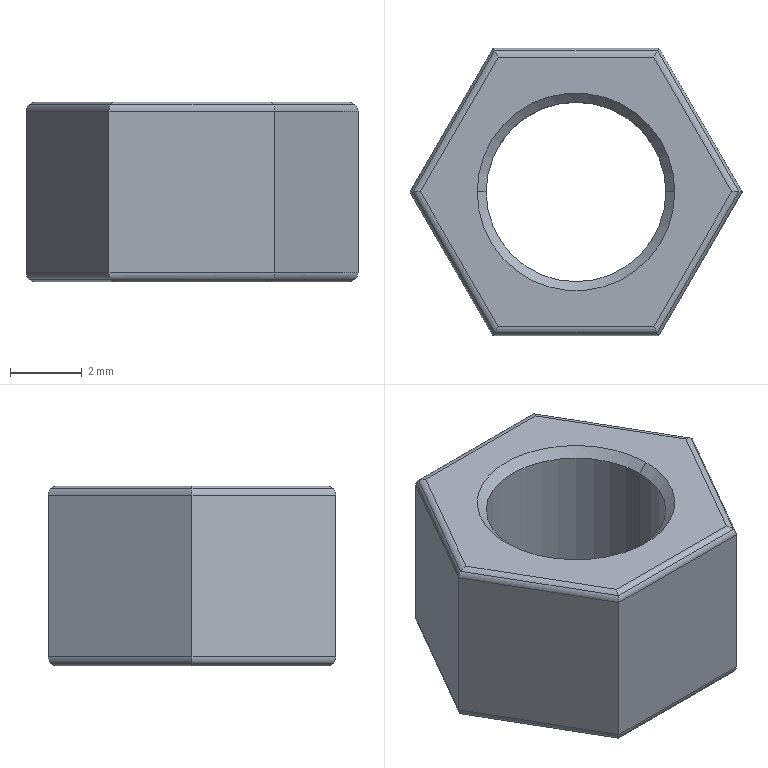Part | SolidWorks | features BaseBody 1 | 1 solid | 38 faces | box 9.238 x 8 x 5 mm | volume 177.206 mm3 | cylinder 26 | plane 8 | cone 4 | commonest cylinder face diameters 0.5 x24 5 x2
STEP:
#1=CARTESIAN_POINT('',(-2.5,0.,0.25));
#2=VERTEX_POINT('',#1);
#3=CARTESIAN_POINT('',(2.5,0.,0.25));
#4=VERTEX_POINT('',#3);
#5=CARTESIAN_POINT('',(0.,0.,0.25));
#6=DIRECTION('',(0.,0.,1.));
#7=DIRECTION('',(-1.,0.,0.));
#8=AXIS2_PLACEMENT_3D('',#5,#6,#7);
#9=CIRCLE('',#8,2.5);
#10=EDGE_CURVE('',#2,#4,#9,.T.);
#11=ORIENTED_EDGE('',*,*,#10,.T.);
#12=CARTESIAN_POINT('',(2.75,0.,0.));
#13=VERTEX_POINT('',#12);
#14=CARTESIAN_POINT('',(2.625,0.,0.125));
#15=DIRECTION('',(0.7071,0.,-0.7071));
#16=VECTOR('',#15,1000.);
#17=LINE('',#14,#16);
#18=EDGE_CURVE('',#4,#13,#17,.T.);
#19=ORIENTED_EDGE('',*,*,#18,.T.);
#20=CARTESIAN_POINT('',(-2.75,0.,0.));
#21=VERTEX_POINT('',#20);
#22=CARTESIAN_POINT('',(0.,0.,0.));
#23=DIRECTION('',(0.,0.,-1.));
#24=DIRECTION('',(-1.,0.,0.));
#25=AXIS2_PLACEMENT_3D('',#22,#23,#24);
#26=CIRCLE('',#25,2.75);
#27=EDGE_CURVE('',#13,#21,#26,.T.);
#28=ORIENTED_EDGE('',*,*,#27,.T.);
#29=CARTESIAN_POINT('',(-2.625,0.,0.125));
#30=DIRECTION('',(-0.7071,0.,-0.7071));
#31=VECTOR('',#30,1000.);
#32=LINE('',#29,#31);
#33=EDGE_CURVE('',#2,#21,#32,.T.);
#34=ORIENTED_EDGE('',*,*,#33,.F.);
#35=EDGE_LOOP('',(#11,#19,#28,#34));
#36=FACE_OUTER_BOUND('',#35,.T.);
#37=CARTESIAN_POINT('',(0.,0.,0.125));
#38=DIRECTION('',(0.,0.,-1.));
#39=DIRECTION('',(-1.,0.,0.));
#40=AXIS2_PLACEMENT_3D('',#37,#38,#39);
#41=CONICAL_SURFACE('',#40,2.625,0.7854);
#42=ADVANCED_FACE('',(#36),#41,.F.);
#43=CARTESIAN_POINT('',(2.5,0.,4.75));
#44=VERTEX_POINT('',#43);
#45=CARTESIAN_POINT('',(-2.5,0.,4.75));
#46=VERTEX_POINT('',#45);
#47=CARTESIAN_POINT('',(0.,0.,4.75));
#48=DIRECTION('',(0.,0.,-1.));
#49=DIRECTION('',(-1.,0.,0.));
#50=AXIS2_PLACEMENT_3D('',#47,#48,#49);
#51=CIRCLE('',#50,2.5);
#52=EDGE_CURVE('',#44,#46,#51,.T.);
#53=ORIENTED_EDGE('',*,*,#52,.F.);
#54=CARTESIAN_POINT('',(2.5,0.,0.));
#55=DIRECTION('',(0.,0.,-1.));
#56=VECTOR('',#55,1000.);
#57=LINE('',#54,#56);
#58=EDGE_CURVE('',#44,#4,#57,.T.);
#59=ORIENTED_EDGE('',*,*,#58,.T.);
#60=ORIENTED_EDGE('',*,*,#10,.F.);
#61=CARTESIAN_POINT('',(-2.5,0.,0.));
#62=DIRECTION('',(0.,0.,-1.));
#63=VECTOR('',#62,1000.);
#64=LINE('',#61,#63);
#65=EDGE_CURVE('',#46,#2,#64,.T.);
#66=ORIENTED_EDGE('',*,*,#65,.F.);
#67=EDGE_LOOP('',(#53,#59,#60,#66));
#68=FACE_OUTER_BOUND('',#67,.T.);
#69=CARTESIAN_POINT('',(0.,0.,0.));
#70=DIRECTION('',(0.,0.,-1.));
#71=DIRECTION('',(-1.,0.,0.));
#72=AXIS2_PLACEMENT_3D('',#69,#70,#71);
#73=CYLINDRICAL_SURFACE('',#72,2.5);
#74=ADVANCED_FACE('',(#68),#73,.F.);
#75=CARTESIAN_POINT('',(0.,0.,4.75));
#76=DIRECTION('',(0.,0.,-1.));
#77=DIRECTION('',(-1.,0.,0.));
#78=AXIS2_PLACEMENT_3D('',#75,#76,#77);
#79=CIRCLE('',#78,2.5);
#80=EDGE_CURVE('',#46,#44,#79,.T.);
#81=ORIENTED_EDGE('',*,*,#80,.T.);
#82=CARTESIAN_POINT('',(2.75,0.,5.));
#83=VERTEX_POINT('',#82);
#84=CARTESIAN_POINT('',(2.625,0.,4.875));
#85=DIRECTION('',(0.7071,0.,0.7071));
#86=VECTOR('',#85,1000.);
#87=LINE('',#84,#86);
#88=EDGE_CURVE('',#44,#83,#87,.T.);
#89=ORIENTED_EDGE('',*,*,#88,.T.);
#90=CARTESIAN_POINT('',(-2.75,0.,5.));
#91=VERTEX_POINT('',#90);
#92=CARTESIAN_POINT('',(0.,0.,5.));
#93=DIRECTION('',(0.,0.,1.));
#94=DIRECTION('',(-1.,0.,0.));
#95=AXIS2_PLACEMENT_3D('',#92,#93,#94);
#96=CIRCLE('',#95,2.75);
#97=EDGE_CURVE('',#83,#91,#96,.T.);
#98=ORIENTED_EDGE('',*,*,#97,.T.);
#99=CARTESIAN_POINT('',(-2.625,0.,4.875));
#100=DIRECTION('',(-0.7071,0.,0.7071));
#101=VECTOR('',#100,1000.);
#102=LINE('',#99,#101);
#103=EDGE_CURVE('',#46,#91,#102,.T.);
#104=ORIENTED_EDGE('',*,*,#103,.F.);
#105=EDGE_LOOP('',(#81,#89,#98,#104));
#106=FACE_OUTER_BOUND('',#105,.T.);
#107=CARTESIAN_POINT('',(0.,0.,4.875));
#108=DIRECTION('',(0.,0.,1.));
#109=DIRECTION('',(-1.,0.,0.));
#110=AXIS2_PLACEMENT_3D('',#107,#108,#109);
#111=CONICAL_SURFACE('',#110,2.625,0.7854);
#112=ADVANCED_FACE('',(#106),#111,.F.);
#113=CARTESIAN_POINT('',(2.309,4.,0.25));
#114=VERTEX_POINT('',#113);
#115=CARTESIAN_POINT('',(2.267,3.927,0.07322));
#116=VERTEX_POINT('',#115);
#117=CARTESIAN_POINT('',(2.309,4.,0.25));
#118=CARTESIAN_POINT('',(2.309,4.,0.1828));
#119=CARTESIAN_POINT('',(2.295,3.974,0.1207));
#120=CARTESIAN_POINT('',(2.267,3.927,0.07322));
#121=(BOUNDED_CURVE()B_SPLINE_CURVE(3,(#117,#118,#119,#120),.UNSPECIFIED.,.F.,.T.)B_SPLINE_CURVE_WITH_KNOTS((4,4),(3.142,3.927),.UNSPECIFIED.)CURVE()GEOMETRIC_REPRESENTATION_ITEM()RATIONAL_B_SPLINE_CURVE((1.,0.9493,0.9493,1.))REPRESENTATION_ITEM(''));
#122=EDGE_CURVE('',#114,#116,#121,.T.);
#123=ORIENTED_EDGE('',*,*,#122,.T.);
#124=CARTESIAN_POINT('',(-2.267,3.927,0.07322));
#125=VERTEX_POINT('',#124);
#126=CARTESIAN_POINT('',(1.155,3.927,0.07322));
#127=DIRECTION('',(-1.,0.,0.));
#128=VECTOR('',#127,1000.);
#129=LINE('',#126,#128);
#130=EDGE_CURVE('',#116,#125,#129,.T.);
#131=ORIENTED_EDGE('',*,*,#130,.T.);
#132=CARTESIAN_POINT('',(-2.309,4.,0.25));
#133=VERTEX_POINT('',#132);
#134=CARTESIAN_POINT('',(-2.309,4.,0.25));
#135=CARTESIAN_POINT('',(-2.309,4.,0.1828));
#136=CARTESIAN_POINT('',(-2.295,3.974,0.1207));
#137=CARTESIAN_POINT('',(-2.267,3.927,0.07322));
#138=(BOUNDED_CURVE()B_SPLINE_CURVE(3,(#134,#135,#136,#137),.UNSPECIFIED.,.F.,.F.)B_SPLINE_CURVE_WITH_KNOTS((4,4),(3.142,3.927),.UNSPECIFIED.)CURVE()GEOMETRIC_REPRESENTATION_ITEM()RATIONAL_B_SPLINE_CURVE((1.,0.9493,0.9493,1.))REPRESENTATION_ITEM(''));
#139=EDGE_CURVE('',#133,#125,#138,.T.);
#140=ORIENTED_EDGE('',*,*,#139,.F.);
#141=CARTESIAN_POINT('',(1.155,4.,0.25));
#142=DIRECTION('',(1.,0.,0.));
#143=VECTOR('',#142,1000.);
#144=LINE('',#141,#143);
#145=EDGE_CURVE('',#133,#114,#144,.T.);
#146=ORIENTED_EDGE('',*,*,#145,.T.);
#147=EDGE_LOOP('',(#123,#131,#140,#146));
#148=FACE_OUTER_BOUND('',#147,.T.);
#149=CARTESIAN_POINT('',(1.155,3.75,0.25));
#150=DIRECTION('',(-1.,0.,0.));
#151=DIRECTION('',(0.,0.7071,-0.7071));
#152=AXIS2_PLACEMENT_3D('',#149,#150,#151);
#153=CYLINDRICAL_SURFACE('',#152,0.25);
#154=ADVANCED_FACE('',(#148),#153,.T.);
#155=CARTESIAN_POINT('',(-2.309,-4.,0.25));
#156=VERTEX_POINT('',#155);
#157=CARTESIAN_POINT('',(-2.267,-3.927,0.07322));
#158=VERTEX_POINT('',#157);
#159=CARTESIAN_POINT('',(-2.309,-4.,0.25));
#160=CARTESIAN_POINT('',(-2.309,-4.,0.1828));
#161=CARTESIAN_POINT('',(-2.295,-3.974,0.1207));
#162=CARTESIAN_POINT('',(-2.267,-3.927,0.07322));
#163=(BOUNDED_CURVE()B_SPLINE_CURVE(3,(#159,#160,#161,#162),.UNSPECIFIED.,.F.,.F.)B_SPLINE_CURVE_WITH_KNOTS((4,4),(3.142,3.927),.UNSPECIFIED.)CURVE()GEOMETRIC_REPRESENTATION_ITEM()RATIONAL_B_SPLINE_CURVE((1.,0.9493,0.9493,1.))REPRESENTATION_ITEM(''));
#164=EDGE_CURVE('',#156,#158,#163,.T.);
#165=ORIENTED_EDGE('',*,*,#164,.T.);
#166=CARTESIAN_POINT('',(2.267,-3.927,0.07322));
#167=VERTEX_POINT('',#166);
#168=CARTESIAN_POINT('',(-1.155,-3.927,0.07322));
#169=DIRECTION('',(1.,0.,0.));
#170=VECTOR('',#169,1000.);
#171=LINE('',#168,#170);
#172=EDGE_CURVE('',#158,#167,#171,.T.);
#173=ORIENTED_EDGE('',*,*,#172,.T.);
#174=CARTESIAN_POINT('',(2.309,-4.,0.25));
#175=VERTEX_POINT('',#174);
#176=CARTESIAN_POINT('',(2.267,-3.927,0.07322));
#177=CARTESIAN_POINT('',(2.295,-3.974,0.1207));
#178=CARTESIAN_POINT('',(2.309,-4.,0.1828));
#179=CARTESIAN_POINT('',(2.309,-4.,0.25));
#180=(BOUNDED_CURVE()B_SPLINE_CURVE(3,(#176,#177,#178,#179),.UNSPECIFIED.,.F.,.F.)B_SPLINE_CURVE_WITH_KNOTS((4,4),(5.498,6.283),.UNSPECIFIED.)CURVE()GEOMETRIC_REPRESENTATION_ITEM()RATIONAL_B_SPLINE_CURVE((1.,0.9493,0.9493,1.))REPRESENTATION_ITEM(''));
#181=EDGE_CURVE('',#167,#175,#180,.T.);
#182=ORIENTED_EDGE('',*,*,#181,.T.);
#183=CARTESIAN_POINT('',(-1.155,-4.,0.25));
#184=DIRECTION('',(-1.,0.,0.));
#185=VECTOR('',#184,1000.);
#186=LINE('',#183,#185);
#187=EDGE_CURVE('',#175,#156,#186,.T.);
#188=ORIENTED_EDGE('',*,*,#187,.T.);
#189=EDGE_LOOP('',(#165,#173,#182,#188));
#190=FACE_OUTER_BOUND('',#189,.T.);
#191=CARTESIAN_POINT('',(-1.155,-3.75,0.25));
#192=DIRECTION('',(1.,0.,0.));
#193=DIRECTION('',(0.,-0.7071,-0.7071));
#194=AXIS2_PLACEMENT_3D('',#191,#192,#193);
#195=CYLINDRICAL_SURFACE('',#194,0.25);
#196=ADVANCED_FACE('',(#190),#195,.T.);
#197=CARTESIAN_POINT('',(4.619,0.,0.25));
#198=VERTEX_POINT('',#197);
#199=CARTESIAN_POINT('',(4.534,0.,0.07322));
#200=VERTEX_POINT('',#199);
#201=CARTESIAN_POINT('',(4.619,0.,0.25));
#202=CARTESIAN_POINT('',(4.619,0.,0.1828));
#203=CARTESIAN_POINT('',(4.589,0.,0.1207));
#204=CARTESIAN_POINT('',(4.534,0.,0.07322));
#205=(BOUNDED_CURVE()B_SPLINE_CURVE(3,(#201,#202,#203,#204),.UNSPECIFIED.,.F.,.F.)B_SPLINE_CURVE_WITH_KNOTS((4,4),(3.142,3.927),.UNSPECIFIED.)CURVE()GEOMETRIC_REPRESENTATION_ITEM()RATIONAL_B_SPLINE_CURVE((1.,0.9493,0.9493,1.))REPRESENTATION_ITEM(''));
#206=EDGE_CURVE('',#198,#200,#205,.T.);
#207=ORIENTED_EDGE('',*,*,#206,.T.);
#208=CARTESIAN_POINT('',(3.978,0.9634,0.07322));
#209=DIRECTION('',(-0.5,0.866,0.));
#210=VECTOR('',#209,1000.);
#211=LINE('',#208,#210);
#212=EDGE_CURVE('',#200,#116,#211,.T.);
#213=ORIENTED_EDGE('',*,*,#212,.T.);
#214=ORIENTED_EDGE('',*,*,#122,.F.);
#215=CARTESIAN_POINT('',(4.041,1.,0.25));
#216=DIRECTION('',(0.5,-0.866,0.));
#217=VECTOR('',#216,1000.);
#218=LINE('',#215,#217);
#219=EDGE_CURVE('',#114,#198,#218,.T.);
#220=ORIENTED_EDGE('',*,*,#219,.T.);
#221=EDGE_LOOP('',(#207,#213,#214,#220));
#222=FACE_OUTER_BOUND('',#221,.T.);
#223=CARTESIAN_POINT('',(3.825,0.875,0.25));
#224=DIRECTION('',(-0.5,0.866,0.));
#225=DIRECTION('',(0.6124,0.3536,-0.7071));
#226=AXIS2_PLACEMENT_3D('',#223,#224,#225);
#227=CYLINDRICAL_SURFACE('',#226,0.25);
#228=ADVANCED_FACE('',(#222),#227,.T.);
#229=ORIENTED_EDGE('',*,*,#181,.F.);
#230=CARTESIAN_POINT('',(2.823,-2.963,0.07322));
#231=DIRECTION('',(0.5,0.866,0.));
#232=VECTOR('',#231,1000.);
#233=LINE('',#230,#232);
#234=EDGE_CURVE('',#167,#200,#233,.T.);
#235=ORIENTED_EDGE('',*,*,#234,.T.);
#236=ORIENTED_EDGE('',*,*,#206,.F.);
#237=CARTESIAN_POINT('',(2.887,-3.,0.25));
#238=DIRECTION('',(-0.5,-0.866,0.));
#239=VECTOR('',#238,1000.);
#240=LINE('',#237,#239);
#241=EDGE_CURVE('',#198,#175,#240,.T.);
#242=ORIENTED_EDGE('',*,*,#241,.T.);
#243=EDGE_LOOP('',(#229,#235,#236,#242));
#244=FACE_OUTER_BOUND('',#243,.T.);
#245=CARTESIAN_POINT('',(2.67,-2.875,0.25));
#246=DIRECTION('',(0.5,0.866,0.));
#247=DIRECTION('',(0.6124,-0.3536,-0.7071));
#248=AXIS2_PLACEMENT_3D('',#245,#246,#247);
#249=CYLINDRICAL_SURFACE('',#248,0.25);
#250=ADVANCED_FACE('',(#244),#249,.T.);
#251=CARTESIAN_POINT('',(-4.619,0.,0.25));
#252=VERTEX_POINT('',#251);
#253=CARTESIAN_POINT('',(-4.534,0.,0.07322));
#254=VERTEX_POINT('',#253);
#255=CARTESIAN_POINT('',(-4.619,0.,0.25));
#256=CARTESIAN_POINT('',(-4.619,0.,0.1828));
#257=CARTESIAN_POINT('',(-4.589,0.,0.1207));
#258=CARTESIAN_POINT('',(-4.534,0.,0.07322));
#259=(BOUNDED_CURVE()B_SPLINE_CURVE(3,(#255,#256,#257,#258),.UNSPECIFIED.,.F.,.T.)B_SPLINE_CURVE_WITH_KNOTS((4,4),(3.142,3.927),.UNSPECIFIED.)CURVE()GEOMETRIC_REPRESENTATION_ITEM()RATIONAL_B_SPLINE_CURVE((1.,0.9493,0.9493,1.))REPRESENTATION_ITEM(''));
#260=EDGE_CURVE('',#252,#254,#259,.T.);
#261=ORIENTED_EDGE('',*,*,#260,.T.);
#262=CARTESIAN_POINT('',(-3.978,-0.9634,0.07322));
#263=DIRECTION('',(0.5,-0.866,0.));
#264=VECTOR('',#263,1000.);
#265=LINE('',#262,#264);
#266=EDGE_CURVE('',#254,#158,#265,.T.);
#267=ORIENTED_EDGE('',*,*,#266,.T.);
#268=ORIENTED_EDGE('',*,*,#164,.F.);
#269=CARTESIAN_POINT('',(-4.041,-1.,0.25));
#270=DIRECTION('',(-0.5,0.866,0.));
#271=VECTOR('',#270,1000.);
#272=LINE('',#269,#271);
#273=EDGE_CURVE('',#156,#252,#272,.T.);
#274=ORIENTED_EDGE('',*,*,#273,.T.);
#275=EDGE_LOOP('',(#261,#267,#268,#274));
#276=FACE_OUTER_BOUND('',#275,.T.);
#277=CARTESIAN_POINT('',(-3.825,-0.875,0.25));
#278=DIRECTION('',(0.5,-0.866,0.));
#279=DIRECTION('',(-0.6124,-0.3536,-0.7071));
#280=AXIS2_PLACEMENT_3D('',#277,#278,#279);
#281=CYLINDRICAL_SURFACE('',#280,0.25);
#282=ADVANCED_FACE('',(#276),#281,.T.);
#283=ORIENTED_EDGE('',*,*,#139,.T.);
#284=CARTESIAN_POINT('',(-2.823,2.963,0.07322));
#285=DIRECTION('',(-0.5,-0.866,0.));
#286=VECTOR('',#285,1000.);
#287=LINE('',#284,#286);
#288=EDGE_CURVE('',#125,#254,#287,.T.);
#289=ORIENTED_EDGE('',*,*,#288,.T.);
#290=ORIENTED_EDGE('',*,*,#260,.F.);
#291=CARTESIAN_POINT('',(-2.887,3.,0.25));
#292=DIRECTION('',(0.5,0.866,0.));
#293=VECTOR('',#292,1000.);
#294=LINE('',#291,#293);
#295=EDGE_CURVE('',#252,#133,#294,.T.);
#296=ORIENTED_EDGE('',*,*,#295,.T.);
#297=EDGE_LOOP('',(#283,#289,#290,#296));
#298=FACE_OUTER_BOUND('',#297,.T.);
#299=CARTESIAN_POINT('',(-2.67,2.875,0.25));
#300=DIRECTION('',(-0.5,-0.866,0.));
#301=DIRECTION('',(-0.6124,0.3536,-0.7071));
#302=AXIS2_PLACEMENT_3D('',#299,#300,#301);
#303=CYLINDRICAL_SURFACE('',#302,0.25);
#304=ADVANCED_FACE('',(#298),#303,.T.);
#305=CARTESIAN_POINT('',(2.267,-3.927,4.927));
#306=VERTEX_POINT('',#305);
#307=CARTESIAN_POINT('',(2.309,-4.,4.75));
#308=VERTEX_POINT('',#307);
#309=CARTESIAN_POINT('',(2.267,-3.927,4.927));
#310=CARTESIAN_POINT('',(2.295,-3.974,4.879));
#311=CARTESIAN_POINT('',(2.309,-4.,4.817));
#312=CARTESIAN_POINT('',(2.309,-4.,4.75));
#313=(BOUNDED_CURVE()B_SPLINE_CURVE(3,(#309,#310,#311,#312),.UNSPECIFIED.,.F.,.F.)B_SPLINE_CURVE_WITH_KNOTS((4,4),(5.498,6.283),.UNSPECIFIED.)CURVE()GEOMETRIC_REPRESENTATION_ITEM()RATIONAL_B_SPLINE_CURVE((1.,0.9493,0.9493,1.))REPRESENTATION_ITEM(''));
#314=EDGE_CURVE('',#306,#308,#313,.T.);
#315=ORIENTED_EDGE('',*,*,#314,.F.);
#316=CARTESIAN_POINT('',(-2.267,-3.927,4.927));
#317=VERTEX_POINT('',#316);
#318=CARTESIAN_POINT('',(-1.155,-3.927,4.927));
#319=DIRECTION('',(-1.,0.,0.));
#320=VECTOR('',#319,1000.);
#321=LINE('',#318,#320);
#322=EDGE_CURVE('',#306,#317,#321,.T.);
#323=ORIENTED_EDGE('',*,*,#322,.T.);
#324=CARTESIAN_POINT('',(-2.309,-4.,4.75));
#325=VERTEX_POINT('',#324);
#326=CARTESIAN_POINT('',(-2.267,-3.927,4.927));
#327=CARTESIAN_POINT('',(-2.295,-3.974,4.879));
#328=CARTESIAN_POINT('',(-2.309,-4.,4.817));
#329=CARTESIAN_POINT('',(-2.309,-4.,4.75));
#330=(BOUNDED_CURVE()B_SPLINE_CURVE(3,(#326,#327,#328,#329),.UNSPECIFIED.,.F.,.F.)B_SPLINE_CURVE_WITH_KNOTS((4,4),(5.498,6.283),.UNSPECIFIED.)CURVE()GEOMETRIC_REPRESENTATION_ITEM()RATIONAL_B_SPLINE_CURVE((1.,0.9493,0.9493,1.))REPRESENTATION_ITEM(''));
#331=EDGE_CURVE('',#317,#325,#330,.T.);
#332=ORIENTED_EDGE('',*,*,#331,.T.);
#333=CARTESIAN_POINT('',(-1.155,-4.,4.75));
#334=DIRECTION('',(1.,0.,0.));
#335=VECTOR('',#334,1000.);
#336=LINE('',#333,#335);
#337=EDGE_CURVE('',#325,#308,#336,.T.);
#338=ORIENTED_EDGE('',*,*,#337,.T.);
#339=EDGE_LOOP('',(#315,#323,#332,#338));
#340=FACE_OUTER_BOUND('',#339,.T.);
#341=CARTESIAN_POINT('',(-1.155,-3.75,4.75));
#342=DIRECTION('',(-1.,0.,0.));
#343=DIRECTION('',(0.,-0.7071,0.7071));
#344=AXIS2_PLACEMENT_3D('',#341,#342,#343);
#345=CYLINDRICAL_SURFACE('',#344,0.25);
#346=ADVANCED_FACE('',(#340),#345,.T.);
#347=ORIENTED_EDGE('',*,*,#331,.F.);
#348=CARTESIAN_POINT('',(-4.534,0.,4.927));
#349=VERTEX_POINT('',#348);
#350=CARTESIAN_POINT('',(-3.978,-0.9634,4.927));
#351=DIRECTION('',(-0.5,0.866,0.));
#352=VECTOR('',#351,1000.);
#353=LINE('',#350,#352);
#354=EDGE_CURVE('',#317,#349,#353,.T.);
#355=ORIENTED_EDGE('',*,*,#354,.T.);
#356=CARTESIAN_POINT('',(-4.619,0.,4.75));
#357=VERTEX_POINT('',#356);
#358=CARTESIAN_POINT('',(-4.534,0.,4.927));
#359=CARTESIAN_POINT('',(-4.589,0.,4.879));
#360=CARTESIAN_POINT('',(-4.619,0.,4.817));
#361=CARTESIAN_POINT('',(-4.619,0.,4.75));
#362=(BOUNDED_CURVE()B_SPLINE_CURVE(3,(#358,#359,#360,#361),.UNSPECIFIED.,.F.,.F.)B_SPLINE_CURVE_WITH_KNOTS((4,4),(5.498,6.283),.UNSPECIFIED.)CURVE()GEOMETRIC_REPRESENTATION_ITEM()RATIONAL_B_SPLINE_CURVE((1.,0.9493,0.9493,1.))REPRESENTATION_ITEM(''));
#363=EDGE_CURVE('',#349,#357,#362,.T.);
#364=ORIENTED_EDGE('',*,*,#363,.T.);
#365=CARTESIAN_POINT('',(-4.041,-1.,4.75));
#366=DIRECTION('',(0.5,-0.866,0.));
#367=VECTOR('',#366,1000.);
#368=LINE('',#365,#367);
#369=EDGE_CURVE('',#357,#325,#368,.T.);
#370=ORIENTED_EDGE('',*,*,#369,.T.);
#371=EDGE_LOOP('',(#347,#355,#364,#370));
#372=FACE_OUTER_BOUND('',#371,.T.);
#373=CARTESIAN_POINT('',(-3.825,-0.875,4.75));
#374=DIRECTION('',(-0.5,0.866,0.));
#375=DIRECTION('',(-0.6124,-0.3536,0.7071));
#376=AXIS2_PLACEMENT_3D('',#373,#374,#375);
#377=CYLINDRICAL_SURFACE('',#376,0.25);
#378=ADVANCED_FACE('',(#372),#377,.T.);
#379=ORIENTED_EDGE('',*,*,#363,.F.);
#380=CARTESIAN_POINT('',(-2.267,3.927,4.927));
#381=VERTEX_POINT('',#380);
#382=CARTESIAN_POINT('',(-2.823,2.963,4.927));
#383=DIRECTION('',(0.5,0.866,0.));
#384=VECTOR('',#383,1000.);
#385=LINE('',#382,#384);
#386=EDGE_CURVE('',#349,#381,#385,.T.);
#387=ORIENTED_EDGE('',*,*,#386,.T.);
#388=CARTESIAN_POINT('',(-2.309,4.,4.75));
#389=VERTEX_POINT('',#388);
#390=CARTESIAN_POINT('',(-2.267,3.927,4.927));
#391=CARTESIAN_POINT('',(-2.295,3.974,4.879));
#392=CARTESIAN_POINT('',(-2.309,4.,4.817));
#393=CARTESIAN_POINT('',(-2.309,4.,4.75));
#394=(BOUNDED_CURVE()B_SPLINE_CURVE(3,(#390,#391,#392,#393),.UNSPECIFIED.,.F.,.F.)B_SPLINE_CURVE_WITH_KNOTS((4,4),(5.498,6.283),.UNSPECIFIED.)CURVE()GEOMETRIC_REPRESENTATION_ITEM()RATIONAL_B_SPLINE_CURVE((1.,0.9493,0.9493,1.))REPRESENTATION_ITEM(''));
#395=EDGE_CURVE('',#381,#389,#394,.T.);
#396=ORIENTED_EDGE('',*,*,#395,.T.);
#397=CARTESIAN_POINT('',(-2.887,3.,4.75));
#398=DIRECTION('',(-0.5,-0.866,0.));
#399=VECTOR('',#398,1000.);
#400=LINE('',#397,#399);
#401=EDGE_CURVE('',#389,#357,#400,.T.);
#402=ORIENTED_EDGE('',*,*,#401,.T.);
#403=EDGE_LOOP('',(#379,#387,#396,#402));
#404=FACE_OUTER_BOUND('',#403,.T.);
#405=CARTESIAN_POINT('',(-2.67,2.875,4.75));
#406=DIRECTION('',(0.5,0.866,0.));
#407=DIRECTION('',(-0.6124,0.3536,0.7071));
#408=AXIS2_PLACEMENT_3D('',#405,#406,#407);
#409=CYLINDRICAL_SURFACE('',#408,0.25);
#410=ADVANCED_FACE('',(#404),#409,.T.);
#411=ORIENTED_EDGE('',*,*,#395,.F.);
#412=CARTESIAN_POINT('',(2.267,3.927,4.927));
#413=VERTEX_POINT('',#412);
#414=CARTESIAN_POINT('',(1.155,3.927,4.927));
#415=DIRECTION('',(1.,0.,0.));
#416=VECTOR('',#415,1000.);
#417=LINE('',#414,#416);
#418=EDGE_CURVE('',#381,#413,#417,.T.);
#419=ORIENTED_EDGE('',*,*,#418,.T.);
#420=CARTESIAN_POINT('',(2.309,4.,4.75));
#421=VERTEX_POINT('',#420);
#422=CARTESIAN_POINT('',(2.267,3.927,4.927));
#423=CARTESIAN_POINT('',(2.295,3.974,4.879));
#424=CARTESIAN_POINT('',(2.309,4.,4.817));
#425=CARTESIAN_POINT('',(2.309,4.,4.75));
#426=(BOUNDED_CURVE()B_SPLINE_CURVE(3,(#422,#423,#424,#425),.UNSPECIFIED.,.F.,.T.)B_SPLINE_CURVE_WITH_KNOTS((4,4),(5.498,6.283),.UNSPECIFIED.)CURVE()GEOMETRIC_REPRESENTATION_ITEM()RATIONAL_B_SPLINE_CURVE((1.,0.9493,0.9493,1.))REPRESENTATION_ITEM(''));
#427=EDGE_CURVE('',#413,#421,#426,.T.);
#428=ORIENTED_EDGE('',*,*,#427,.T.);
#429=CARTESIAN_POINT('',(1.155,4.,4.75));
#430=DIRECTION('',(-1.,0.,0.));
#431=VECTOR('',#430,1000.);
#432=LINE('',#429,#431);
#433=EDGE_CURVE('',#421,#389,#432,.T.);
#434=ORIENTED_EDGE('',*,*,#433,.T.);
#435=EDGE_LOOP('',(#411,#419,#428,#434));
#436=FACE_OUTER_BOUND('',#435,.T.);
#437=CARTESIAN_POINT('',(1.155,3.75,4.75));
#438=DIRECTION('',(1.,0.,0.));
#439=DIRECTION('',(0.,0.7071,0.7071));
#440=AXIS2_PLACEMENT_3D('',#437,#438,#439);
#441=CYLINDRICAL_SURFACE('',#440,0.25);
#442=ADVANCED_FACE('',(#436),#441,.T.);
#443=ORIENTED_EDGE('',*,*,#427,.F.);
#444=CARTESIAN_POINT('',(4.534,0.,4.927));
#445=VERTEX_POINT('',#444);
#446=CARTESIAN_POINT('',(3.978,0.9634,4.927));
#447=DIRECTION('',(0.5,-0.866,0.));
#448=VECTOR('',#447,1000.);
#449=LINE('',#446,#448);
#450=EDGE_CURVE('',#413,#445,#449,.T.);
#451=ORIENTED_EDGE('',*,*,#450,.T.);
#452=CARTESIAN_POINT('',(4.619,0.,4.75));
#453=VERTEX_POINT('',#452);
#454=CARTESIAN_POINT('',(4.534,0.,4.927));
#455=CARTESIAN_POINT('',(4.589,0.,4.879));
#456=CARTESIAN_POINT('',(4.619,0.,4.817));
#457=CARTESIAN_POINT('',(4.619,0.,4.75));
#458=(BOUNDED_CURVE()B_SPLINE_CURVE(3,(#454,#455,#456,#457),.UNSPECIFIED.,.F.,.T.)B_SPLINE_CURVE_WITH_KNOTS((4,4),(5.498,6.283),.UNSPECIFIED.)CURVE()GEOMETRIC_REPRESENTATION_ITEM()RATIONAL_B_SPLINE_CURVE((1.,0.9493,0.9493,1.))REPRESENTATION_ITEM(''));
#459=EDGE_CURVE('',#445,#453,#458,.T.);
#460=ORIENTED_EDGE('',*,*,#459,.T.);
#461=CARTESIAN_POINT('',(4.041,1.,4.75));
#462=DIRECTION('',(-0.5,0.866,0.));
#463=VECTOR('',#462,1000.);
#464=LINE('',#461,#463);
#465=EDGE_CURVE('',#453,#421,#464,.T.);
#466=ORIENTED_EDGE('',*,*,#465,.T.);
#467=EDGE_LOOP('',(#443,#451,#460,#466));
#468=FACE_OUTER_BOUND('',#467,.T.);
#469=CARTESIAN_POINT('',(3.825,0.875,4.75));
#470=DIRECTION('',(0.5,-0.866,0.));
#471=DIRECTION('',(0.6124,0.3536,0.7071));
#472=AXIS2_PLACEMENT_3D('',#469,#470,#471);
#473=CYLINDRICAL_SURFACE('',#472,0.25);
#474=ADVANCED_FACE('',(#468),#473,.T.);
#475=ORIENTED_EDGE('',*,*,#459,.F.);
#476=CARTESIAN_POINT('',(2.823,-2.963,4.927));
#477=DIRECTION('',(-0.5,-0.866,0.));
#478=VECTOR('',#477,1000.);
#479=LINE('',#476,#478);
#480=EDGE_CURVE('',#445,#306,#479,.T.);
#481=ORIENTED_EDGE('',*,*,#480,.T.);
#482=ORIENTED_EDGE('',*,*,#314,.T.);
#483=CARTESIAN_POINT('',(2.887,-3.,4.75));
#484=DIRECTION('',(0.5,0.866,0.));
#485=VECTOR('',#484,1000.);
#486=LINE('',#483,#485);
#487=EDGE_CURVE('',#308,#453,#486,.T.);
#488=ORIENTED_EDGE('',*,*,#487,.T.);
#489=EDGE_LOOP('',(#475,#481,#482,#488));
#490=FACE_OUTER_BOUND('',#489,.T.);
#491=CARTESIAN_POINT('',(2.67,-2.875,4.75));
#492=DIRECTION('',(-0.5,-0.866,0.));
#493=DIRECTION('',(0.6124,-0.3536,0.7071));
#494=AXIS2_PLACEMENT_3D('',#491,#492,#493);
#495=CYLINDRICAL_SURFACE('',#494,0.25);
#496=ADVANCED_FACE('',(#490),#495,.T.);
#497=CARTESIAN_POINT('',(0.,0.,0.));
#498=DIRECTION('',(0.,0.,-1.));
#499=DIRECTION('',(-1.,0.,0.));
#500=AXIS2_PLACEMENT_3D('',#497,#498,#499);
#501=CIRCLE('',#500,2.75);
#502=EDGE_CURVE('',#21,#13,#501,.T.);
#503=ORIENTED_EDGE('',*,*,#502,.F.);
#504=ORIENTED_EDGE('',*,*,#27,.F.);
#505=EDGE_LOOP('',(#503,#504));
#506=FACE_BOUND('',#505,.T.);
#507=CARTESIAN_POINT('',(-2.165,-3.75,0.));
#508=VERTEX_POINT('',#507);
#509=CARTESIAN_POINT('',(2.165,-3.75,0.));
#510=VERTEX_POINT('',#509);
#511=CARTESIAN_POINT('',(-1.155,-3.75,0.));
#512=DIRECTION('',(1.,0.,0.));
#513=VECTOR('',#512,1000.);
#514=LINE('',#511,#513);
#515=EDGE_CURVE('',#508,#510,#514,.T.);
#516=ORIENTED_EDGE('',*,*,#515,.F.);
#517=CARTESIAN_POINT('',(-4.33,0.,0.));
#518=VERTEX_POINT('',#517);
#519=CARTESIAN_POINT('',(-3.825,-0.875,0.));
#520=DIRECTION('',(0.5,-0.866,0.));
#521=VECTOR('',#520,1000.);
#522=LINE('',#519,#521);
#523=EDGE_CURVE('',#518,#508,#522,.T.);
#524=ORIENTED_EDGE('',*,*,#523,.F.);
#525=CARTESIAN_POINT('',(-2.165,3.75,0.));
#526=VERTEX_POINT('',#525);
#527=CARTESIAN_POINT('',(-2.67,2.875,0.));
#528=DIRECTION('',(-0.5,-0.866,0.));
#529=VECTOR('',#528,1000.);
#530=LINE('',#527,#529);
#531=EDGE_CURVE('',#526,#518,#530,.T.);
#532=ORIENTED_EDGE('',*,*,#531,.F.);
#533=CARTESIAN_POINT('',(2.165,3.75,0.));
#534=VERTEX_POINT('',#533);
#535=CARTESIAN_POINT('',(1.155,3.75,0.));
#536=DIRECTION('',(-1.,0.,0.));
#537=VECTOR('',#536,1000.);
#538=LINE('',#535,#537);
#539=EDGE_CURVE('',#534,#526,#538,.T.);
#540=ORIENTED_EDGE('',*,*,#539,.F.);
#541=CARTESIAN_POINT('',(4.33,0.,0.));
#542=VERTEX_POINT('',#541);
#543=CARTESIAN_POINT('',(3.825,0.875,0.));
#544=DIRECTION('',(-0.5,0.866,0.));
#545=VECTOR('',#544,1000.);
#546=LINE('',#543,#545);
#547=EDGE_CURVE('',#542,#534,#546,.T.);
#548=ORIENTED_EDGE('',*,*,#547,.F.);
#549=CARTESIAN_POINT('',(2.67,-2.875,0.));
#550=DIRECTION('',(0.5,0.866,0.));
#551=VECTOR('',#550,1000.);
#552=LINE('',#549,#551);
#553=EDGE_CURVE('',#510,#542,#552,.T.);
#554=ORIENTED_EDGE('',*,*,#553,.F.);
#555=EDGE_LOOP('',(#516,#524,#532,#540,#548,#554));
#556=FACE_OUTER_BOUND('',#555,.T.);
#557=CARTESIAN_POINT('',(0.,0.,0.));
#558=DIRECTION('',(0.,0.,1.));
#559=DIRECTION('',(1.,0.,0.));
#560=AXIS2_PLACEMENT_3D('',#557,#558,#559);
#561=PLANE('',#560);
#562=ADVANCED_FACE('',(#506,#556),#561,.F.);
#563=CARTESIAN_POINT('',(0.,0.,5.));
#564=DIRECTION('',(0.,0.,1.));
#565=DIRECTION('',(-1.,0.,0.));
#566=AXIS2_PLACEMENT_3D('',#563,#564,#565);
#567=CIRCLE('',#566,2.75);
#568=EDGE_CURVE('',#91,#83,#567,.T.);
#569=ORIENTED_EDGE('',*,*,#568,.F.);
#570=ORIENTED_EDGE('',*,*,#97,.F.);
#571=EDGE_LOOP('',(#569,#570));
#572=FACE_BOUND('',#571,.T.);
#573=CARTESIAN_POINT('',(2.165,-3.75,5.));
#574=VERTEX_POINT('',#573);
#575=CARTESIAN_POINT('',(-2.165,-3.75,5.));
#576=VERTEX_POINT('',#575);
#577=CARTESIAN_POINT('',(-1.155,-3.75,5.));
#578=DIRECTION('',(-1.,0.,0.));
#579=VECTOR('',#578,1000.);
#580=LINE('',#577,#579);
#581=EDGE_CURVE('',#574,#576,#580,.T.);
#582=ORIENTED_EDGE('',*,*,#581,.F.);
#583=CARTESIAN_POINT('',(4.33,0.,5.));
#584=VERTEX_POINT('',#583);
#585=CARTESIAN_POINT('',(2.67,-2.875,5.));
#586=DIRECTION('',(-0.5,-0.866,0.));
#587=VECTOR('',#586,1000.);
#588=LINE('',#585,#587);
#589=EDGE_CURVE('',#584,#574,#588,.T.);
#590=ORIENTED_EDGE('',*,*,#589,.F.);
#591=CARTESIAN_POINT('',(2.165,3.75,5.));
#592=VERTEX_POINT('',#591);
#593=CARTESIAN_POINT('',(3.825,0.875,5.));
#594=DIRECTION('',(0.5,-0.866,0.));
#595=VECTOR('',#594,1000.);
#596=LINE('',#593,#595);
#597=EDGE_CURVE('',#592,#584,#596,.T.);
#598=ORIENTED_EDGE('',*,*,#597,.F.);
#599=CARTESIAN_POINT('',(-2.165,3.75,5.));
#600=VERTEX_POINT('',#599);
#601=CARTESIAN_POINT('',(1.155,3.75,5.));
#602=DIRECTION('',(1.,0.,0.));
#603=VECTOR('',#602,1000.);
#604=LINE('',#601,#603);
#605=EDGE_CURVE('',#600,#592,#604,.T.);
#606=ORIENTED_EDGE('',*,*,#605,.F.);
#607=CARTESIAN_POINT('',(-4.33,0.,5.));
#608=VERTEX_POINT('',#607);
#609=CARTESIAN_POINT('',(-2.67,2.875,5.));
#610=DIRECTION('',(0.5,0.866,0.));
#611=VECTOR('',#610,1000.);
#612=LINE('',#609,#611);
#613=EDGE_CURVE('',#608,#600,#612,.T.);
#614=ORIENTED_EDGE('',*,*,#613,.F.);
#615=CARTESIAN_POINT('',(-3.825,-0.875,5.));
#616=DIRECTION('',(-0.5,0.866,0.));
#617=VECTOR('',#616,1000.);
#618=LINE('',#615,#617);
#619=EDGE_CURVE('',#576,#608,#618,.T.);
#620=ORIENTED_EDGE('',*,*,#619,.F.);
#621=EDGE_LOOP('',(#582,#590,#598,#606,#614,#620));
#622=FACE_OUTER_BOUND('',#621,.T.);
#623=CARTESIAN_POINT('',(0.,0.,5.));
#624=DIRECTION('',(0.,0.,1.));
#625=DIRECTION('',(1.,0.,0.));
#626=AXIS2_PLACEMENT_3D('',#623,#624,#625);
#627=PLANE('',#626);
#628=ADVANCED_FACE('',(#572,#622),#627,.T.);
#629=ORIENTED_EDGE('',*,*,#295,.F.);
#630=CARTESIAN_POINT('',(-4.619,0.,0.));
#631=DIRECTION('',(0.,0.,1.));
#632=VECTOR('',#631,1000.);
#633=LINE('',#630,#632);
#634=EDGE_CURVE('',#252,#357,#633,.T.);
#635=ORIENTED_EDGE('',*,*,#634,.T.);
#636=ORIENTED_EDGE('',*,*,#401,.F.);
#637=CARTESIAN_POINT('',(-2.309,4.,0.));
#638=DIRECTION('',(0.,0.,1.));
#639=VECTOR('',#638,1000.);
#640=LINE('',#637,#639);
#641=EDGE_CURVE('',#133,#389,#640,.T.);
#642=ORIENTED_EDGE('',*,*,#641,.F.);
#643=EDGE_LOOP('',(#629,#635,#636,#642));
#644=FACE_OUTER_BOUND('',#643,.T.);
#645=CARTESIAN_POINT('',(-2.309,4.,0.));
#646=DIRECTION('',(-0.866,0.5,0.));
#647=DIRECTION('',(0.,0.,1.));
#648=AXIS2_PLACEMENT_3D('',#645,#646,#647);
#649=PLANE('',#648);
#650=ADVANCED_FACE('',(#644),#649,.T.);
#651=ORIENTED_EDGE('',*,*,#273,.F.);
#652=CARTESIAN_POINT('',(-2.309,-4.,0.));
#653=DIRECTION('',(0.,0.,1.));
#654=VECTOR('',#653,1000.);
#655=LINE('',#652,#654);
#656=EDGE_CURVE('',#156,#325,#655,.T.);
#657=ORIENTED_EDGE('',*,*,#656,.T.);
#658=ORIENTED_EDGE('',*,*,#369,.F.);
#659=ORIENTED_EDGE('',*,*,#634,.F.);
#660=EDGE_LOOP('',(#651,#657,#658,#659));
#661=FACE_OUTER_BOUND('',#660,.T.);
#662=CARTESIAN_POINT('',(-4.619,0.,0.));
#663=DIRECTION('',(-0.866,-0.5,0.));
#664=DIRECTION('',(-0.5,0.866,0.));
#665=AXIS2_PLACEMENT_3D('',#662,#663,#664);
#666=PLANE('',#665);
#667=ADVANCED_FACE('',(#661),#666,.T.);
#668=ORIENTED_EDGE('',*,*,#187,.F.);
#669=CARTESIAN_POINT('',(2.309,-4.,0.));
#670=DIRECTION('',(0.,0.,1.));
#671=VECTOR('',#670,1000.);
#672=LINE('',#669,#671);
#673=EDGE_CURVE('',#175,#308,#672,.T.);
#674=ORIENTED_EDGE('',*,*,#673,.T.);
#675=ORIENTED_EDGE('',*,*,#337,.F.);
#676=ORIENTED_EDGE('',*,*,#656,.F.);
#677=EDGE_LOOP('',(#668,#674,#675,#676));
#678=FACE_OUTER_BOUND('',#677,.T.);
#679=CARTESIAN_POINT('',(-2.309,-4.,0.));
#680=DIRECTION('',(0.,-1.,0.));
#681=DIRECTION('',(-1.,0.,0.));
#682=AXIS2_PLACEMENT_3D('',#679,#680,#681);
#683=PLANE('',#682);
#684=ADVANCED_FACE('',(#678),#683,.T.);
#685=ORIENTED_EDGE('',*,*,#219,.F.);
#686=CARTESIAN_POINT('',(2.309,4.,0.));
#687=DIRECTION('',(0.,0.,1.));
#688=VECTOR('',#687,1000.);
#689=LINE('',#686,#688);
#690=EDGE_CURVE('',#114,#421,#689,.T.);
#691=ORIENTED_EDGE('',*,*,#690,.T.);
#692=ORIENTED_EDGE('',*,*,#465,.F.);
#693=CARTESIAN_POINT('',(4.619,0.,0.));
#694=DIRECTION('',(0.,0.,1.));
#695=VECTOR('',#694,1000.);
#696=LINE('',#693,#695);
#697=EDGE_CURVE('',#198,#453,#696,.T.);
#698=ORIENTED_EDGE('',*,*,#697,.F.);
#699=EDGE_LOOP('',(#685,#691,#692,#698));
#700=FACE_OUTER_BOUND('',#699,.T.);
#701=CARTESIAN_POINT('',(4.619,0.,0.));
#702=DIRECTION('',(0.866,0.5,0.));
#703=DIRECTION('',(0.,0.,-1.));
#704=AXIS2_PLACEMENT_3D('',#701,#702,#703);
#705=PLANE('',#704);
#706=ADVANCED_FACE('',(#700),#705,.T.);
#707=ORIENTED_EDGE('',*,*,#241,.F.);
#708=ORIENTED_EDGE('',*,*,#697,.T.);
#709=ORIENTED_EDGE('',*,*,#487,.F.);
#710=ORIENTED_EDGE('',*,*,#673,.F.);
#711=EDGE_LOOP('',(#707,#708,#709,#710));
#712=FACE_OUTER_BOUND('',#711,.T.);
#713=CARTESIAN_POINT('',(2.309,-4.,0.));
#714=DIRECTION('',(0.866,-0.5,0.));
#715=DIRECTION('',(0.,0.,-1.));
#716=AXIS2_PLACEMENT_3D('',#713,#714,#715);
#717=PLANE('',#716);
#718=ADVANCED_FACE('',(#712),#717,.T.);
#719=ORIENTED_EDGE('',*,*,#145,.F.);
#720=ORIENTED_EDGE('',*,*,#641,.T.);
#721=ORIENTED_EDGE('',*,*,#433,.F.);
#722=ORIENTED_EDGE('',*,*,#690,.F.);
#723=EDGE_LOOP('',(#719,#720,#721,#722));
#724=FACE_OUTER_BOUND('',#723,.T.);
#725=CARTESIAN_POINT('',(2.309,4.,0.));
#726=DIRECTION('',(0.,1.,0.));
#727=DIRECTION('',(1.,0.,0.));
#728=AXIS2_PLACEMENT_3D('',#725,#726,#727);
#729=PLANE('',#728);
#730=ADVANCED_FACE('',(#724),#729,.T.);
#731=ORIENTED_EDGE('',*,*,#480,.F.);
#732=CARTESIAN_POINT('',(4.33,0.,5.));
#733=CARTESIAN_POINT('',(4.408,0.,5.));
#734=CARTESIAN_POINT('',(4.479,0.,4.974));
#735=CARTESIAN_POINT('',(4.534,0.,4.927));
#736=(BOUNDED_CURVE()B_SPLINE_CURVE(3,(#732,#733,#734,#735),.UNSPECIFIED.,.F.,.F.)B_SPLINE_CURVE_WITH_KNOTS((4,4),(4.712,5.498),.UNSPECIFIED.)CURVE()GEOMETRIC_REPRESENTATION_ITEM()RATIONAL_B_SPLINE_CURVE((1.,0.9493,0.9493,1.))REPRESENTATION_ITEM(''));
#737=EDGE_CURVE('',#584,#445,#736,.T.);
#738=ORIENTED_EDGE('',*,*,#737,.F.);
#739=ORIENTED_EDGE('',*,*,#589,.T.);
#740=CARTESIAN_POINT('',(2.165,-3.75,5.));
#741=CARTESIAN_POINT('',(2.204,-3.817,5.));
#742=CARTESIAN_POINT('',(2.24,-3.879,4.974));
#743=CARTESIAN_POINT('',(2.267,-3.927,4.927));
#744=(BOUNDED_CURVE()B_SPLINE_CURVE(3,(#740,#741,#742,#743),.UNSPECIFIED.,.F.,.F.)B_SPLINE_CURVE_WITH_KNOTS((4,4),(4.712,5.498),.UNSPECIFIED.)CURVE()GEOMETRIC_REPRESENTATION_ITEM()RATIONAL_B_SPLINE_CURVE((1.,0.9493,0.9493,1.))REPRESENTATION_ITEM(''));
#745=EDGE_CURVE('',#574,#306,#744,.T.);
#746=ORIENTED_EDGE('',*,*,#745,.T.);
#747=EDGE_LOOP('',(#731,#738,#739,#746));
#748=FACE_OUTER_BOUND('',#747,.T.);
#749=CARTESIAN_POINT('',(2.67,-2.875,4.75));
#750=DIRECTION('',(-0.5,-0.866,0.));
#751=DIRECTION('',(0.6124,-0.3536,0.7071));
#752=AXIS2_PLACEMENT_3D('',#749,#750,#751);
#753=CYLINDRICAL_SURFACE('',#752,0.25);
#754=ADVANCED_FACE('',(#748),#753,.T.);
#755=ORIENTED_EDGE('',*,*,#450,.F.);
#756=CARTESIAN_POINT('',(2.165,3.75,5.));
#757=CARTESIAN_POINT('',(2.204,3.817,5.));
#758=CARTESIAN_POINT('',(2.24,3.879,4.974));
#759=CARTESIAN_POINT('',(2.267,3.927,4.927));
#760=(BOUNDED_CURVE()B_SPLINE_CURVE(3,(#756,#757,#758,#759),.UNSPECIFIED.,.F.,.F.)B_SPLINE_CURVE_WITH_KNOTS((4,4),(4.712,5.498),.UNSPECIFIED.)CURVE()GEOMETRIC_REPRESENTATION_ITEM()RATIONAL_B_SPLINE_CURVE((1.,0.9493,0.9493,1.))REPRESENTATION_ITEM(''));
#761=EDGE_CURVE('',#592,#413,#760,.T.);
#762=ORIENTED_EDGE('',*,*,#761,.F.);
#763=ORIENTED_EDGE('',*,*,#597,.T.);
#764=ORIENTED_EDGE('',*,*,#737,.T.);
#765=EDGE_LOOP('',(#755,#762,#763,#764));
#766=FACE_OUTER_BOUND('',#765,.T.);
#767=CARTESIAN_POINT('',(3.825,0.875,4.75));
#768=DIRECTION('',(0.5,-0.866,0.));
#769=DIRECTION('',(0.6124,0.3536,0.7071));
#770=AXIS2_PLACEMENT_3D('',#767,#768,#769);
#771=CYLINDRICAL_SURFACE('',#770,0.25);
#772=ADVANCED_FACE('',(#766),#771,.T.);
#773=ORIENTED_EDGE('',*,*,#418,.F.);
#774=CARTESIAN_POINT('',(-2.165,3.75,5.));
#775=CARTESIAN_POINT('',(-2.204,3.817,5.));
#776=CARTESIAN_POINT('',(-2.24,3.879,4.974));
#777=CARTESIAN_POINT('',(-2.267,3.927,4.927));
#778=(BOUNDED_CURVE()B_SPLINE_CURVE(3,(#774,#775,#776,#777),.UNSPECIFIED.,.F.,.T.)B_SPLINE_CURVE_WITH_KNOTS((4,4),(4.712,5.498),.UNSPECIFIED.)CURVE()GEOMETRIC_REPRESENTATION_ITEM()RATIONAL_B_SPLINE_CURVE((1.,0.9493,0.9493,1.))REPRESENTATION_ITEM(''));
#779=EDGE_CURVE('',#600,#381,#778,.T.);
#780=ORIENTED_EDGE('',*,*,#779,.F.);
#781=ORIENTED_EDGE('',*,*,#605,.T.);
#782=ORIENTED_EDGE('',*,*,#761,.T.);
#783=EDGE_LOOP('',(#773,#780,#781,#782));
#784=FACE_OUTER_BOUND('',#783,.T.);
#785=CARTESIAN_POINT('',(1.155,3.75,4.75));
#786=DIRECTION('',(1.,0.,0.));
#787=DIRECTION('',(0.,0.7071,0.7071));
#788=AXIS2_PLACEMENT_3D('',#785,#786,#787);
#789=CYLINDRICAL_SURFACE('',#788,0.25);
#790=ADVANCED_FACE('',(#784),#789,.T.);
#791=ORIENTED_EDGE('',*,*,#386,.F.);
#792=CARTESIAN_POINT('',(-4.33,0.,5.));
#793=CARTESIAN_POINT('',(-4.408,0.,5.));
#794=CARTESIAN_POINT('',(-4.479,0.,4.974));
#795=CARTESIAN_POINT('',(-4.534,0.,4.927));
#796=(BOUNDED_CURVE()B_SPLINE_CURVE(3,(#792,#793,#794,#795),.UNSPECIFIED.,.F.,.F.)B_SPLINE_CURVE_WITH_KNOTS((4,4),(4.712,5.498),.UNSPECIFIED.)CURVE()GEOMETRIC_REPRESENTATION_ITEM()RATIONAL_B_SPLINE_CURVE((1.,0.9493,0.9493,1.))REPRESENTATION_ITEM(''));
#797=EDGE_CURVE('',#608,#349,#796,.T.);
#798=ORIENTED_EDGE('',*,*,#797,.F.);
#799=ORIENTED_EDGE('',*,*,#613,.T.);
#800=ORIENTED_EDGE('',*,*,#779,.T.);
#801=EDGE_LOOP('',(#791,#798,#799,#800));
#802=FACE_OUTER_BOUND('',#801,.T.);
#803=CARTESIAN_POINT('',(-2.67,2.875,4.75));
#804=DIRECTION('',(0.5,0.866,0.));
#805=DIRECTION('',(-0.6124,0.3536,0.7071));
#806=AXIS2_PLACEMENT_3D('',#803,#804,#805);
#807=CYLINDRICAL_SURFACE('',#806,0.25);
#808=ADVANCED_FACE('',(#802),#807,.T.);
#809=ORIENTED_EDGE('',*,*,#354,.F.);
#810=CARTESIAN_POINT('',(-2.165,-3.75,5.));
#811=CARTESIAN_POINT('',(-2.204,-3.817,5.));
#812=CARTESIAN_POINT('',(-2.24,-3.879,4.974));
#813=CARTESIAN_POINT('',(-2.267,-3.927,4.927));
#814=(BOUNDED_CURVE()B_SPLINE_CURVE(3,(#810,#811,#812,#813),.UNSPECIFIED.,.F.,.F.)B_SPLINE_CURVE_WITH_KNOTS((4,4),(4.712,5.498),.UNSPECIFIED.)CURVE()GEOMETRIC_REPRESENTATION_ITEM()RATIONAL_B_SPLINE_CURVE((1.,0.9493,0.9493,1.))REPRESENTATION_ITEM(''));
#815=EDGE_CURVE('',#576,#317,#814,.T.);
#816=ORIENTED_EDGE('',*,*,#815,.F.);
#817=ORIENTED_EDGE('',*,*,#619,.T.);
#818=ORIENTED_EDGE('',*,*,#797,.T.);
#819=EDGE_LOOP('',(#809,#816,#817,#818));
#820=FACE_OUTER_BOUND('',#819,.T.);
#821=CARTESIAN_POINT('',(-3.825,-0.875,4.75));
#822=DIRECTION('',(-0.5,0.866,0.));
#823=DIRECTION('',(-0.6124,-0.3536,0.7071));
#824=AXIS2_PLACEMENT_3D('',#821,#822,#823);
#825=CYLINDRICAL_SURFACE('',#824,0.25);
#826=ADVANCED_FACE('',(#820),#825,.T.);
#827=ORIENTED_EDGE('',*,*,#322,.F.);
#828=ORIENTED_EDGE('',*,*,#745,.F.);
#829=ORIENTED_EDGE('',*,*,#581,.T.);
#830=ORIENTED_EDGE('',*,*,#815,.T.);
#831=EDGE_LOOP('',(#827,#828,#829,#830));
#832=FACE_OUTER_BOUND('',#831,.T.);
#833=CARTESIAN_POINT('',(-1.155,-3.75,4.75));
#834=DIRECTION('',(-1.,0.,0.));
#835=DIRECTION('',(0.,-0.7071,0.7071));
#836=AXIS2_PLACEMENT_3D('',#833,#834,#835);
#837=CYLINDRICAL_SURFACE('',#836,0.25);
#838=ADVANCED_FACE('',(#832),#837,.T.);
#839=ORIENTED_EDGE('',*,*,#288,.F.);
#840=CARTESIAN_POINT('',(-2.267,3.927,0.07322));
#841=CARTESIAN_POINT('',(-2.24,3.879,0.02571));
#842=CARTESIAN_POINT('',(-2.204,3.817,0.));
#843=CARTESIAN_POINT('',(-2.165,3.75,0.));
#844=(BOUNDED_CURVE()B_SPLINE_CURVE(3,(#840,#841,#842,#843),.UNSPECIFIED.,.F.,.T.)B_SPLINE_CURVE_WITH_KNOTS((4,4),(3.927,4.712),.UNSPECIFIED.)CURVE()GEOMETRIC_REPRESENTATION_ITEM()RATIONAL_B_SPLINE_CURVE((1.,0.9493,0.9493,1.))REPRESENTATION_ITEM(''));
#845=EDGE_CURVE('',#125,#526,#844,.T.);
#846=ORIENTED_EDGE('',*,*,#845,.T.);
#847=ORIENTED_EDGE('',*,*,#531,.T.);
#848=CARTESIAN_POINT('',(-4.534,0.,0.07322));
#849=CARTESIAN_POINT('',(-4.479,0.,0.02571));
#850=CARTESIAN_POINT('',(-4.408,0.,0.));
#851=CARTESIAN_POINT('',(-4.33,0.,0.));
#852=(BOUNDED_CURVE()B_SPLINE_CURVE(3,(#848,#849,#850,#851),.UNSPECIFIED.,.F.,.F.)B_SPLINE_CURVE_WITH_KNOTS((4,4),(3.927,4.712),.UNSPECIFIED.)CURVE()GEOMETRIC_REPRESENTATION_ITEM()RATIONAL_B_SPLINE_CURVE((1.,0.9493,0.9493,1.))REPRESENTATION_ITEM(''));
#853=EDGE_CURVE('',#254,#518,#852,.T.);
#854=ORIENTED_EDGE('',*,*,#853,.F.);
#855=EDGE_LOOP('',(#839,#846,#847,#854));
#856=FACE_OUTER_BOUND('',#855,.T.);
#857=CARTESIAN_POINT('',(-2.67,2.875,0.25));
#858=DIRECTION('',(-0.5,-0.866,0.));
#859=DIRECTION('',(-0.6124,0.3536,-0.7071));
#860=AXIS2_PLACEMENT_3D('',#857,#858,#859);
#861=CYLINDRICAL_SURFACE('',#860,0.25);
#862=ADVANCED_FACE('',(#856),#861,.T.);
#863=ORIENTED_EDGE('',*,*,#266,.F.);
#864=ORIENTED_EDGE('',*,*,#853,.T.);
#865=ORIENTED_EDGE('',*,*,#523,.T.);
#866=CARTESIAN_POINT('',(-2.267,-3.927,0.07322));
#867=CARTESIAN_POINT('',(-2.24,-3.879,0.02571));
#868=CARTESIAN_POINT('',(-2.204,-3.817,0.));
#869=CARTESIAN_POINT('',(-2.165,-3.75,0.));
#870=(BOUNDED_CURVE()B_SPLINE_CURVE(3,(#866,#867,#868,#869),.UNSPECIFIED.,.F.,.T.)B_SPLINE_CURVE_WITH_KNOTS((4,4),(3.927,4.712),.UNSPECIFIED.)CURVE()GEOMETRIC_REPRESENTATION_ITEM()RATIONAL_B_SPLINE_CURVE((1.,0.9493,0.9493,1.))REPRESENTATION_ITEM(''));
#871=EDGE_CURVE('',#158,#508,#870,.T.);
#872=ORIENTED_EDGE('',*,*,#871,.F.);
#873=EDGE_LOOP('',(#863,#864,#865,#872));
#874=FACE_OUTER_BOUND('',#873,.T.);
#875=CARTESIAN_POINT('',(-3.825,-0.875,0.25));
#876=DIRECTION('',(0.5,-0.866,0.));
#877=DIRECTION('',(-0.6124,-0.3536,-0.7071));
#878=AXIS2_PLACEMENT_3D('',#875,#876,#877);
#879=CYLINDRICAL_SURFACE('',#878,0.25);
#880=ADVANCED_FACE('',(#874),#879,.T.);
#881=ORIENTED_EDGE('',*,*,#234,.F.);
#882=CARTESIAN_POINT('',(2.165,-3.75,0.));
#883=CARTESIAN_POINT('',(2.204,-3.817,0.));
#884=CARTESIAN_POINT('',(2.24,-3.879,0.02571));
#885=CARTESIAN_POINT('',(2.267,-3.927,0.07322));
#886=(BOUNDED_CURVE()B_SPLINE_CURVE(3,(#882,#883,#884,#885),.UNSPECIFIED.,.F.,.F.)B_SPLINE_CURVE_WITH_KNOTS((4,4),(4.712,5.498),.UNSPECIFIED.)CURVE()GEOMETRIC_REPRESENTATION_ITEM()RATIONAL_B_SPLINE_CURVE((1.,0.9493,0.9493,1.))REPRESENTATION_ITEM(''));
#887=EDGE_CURVE('',#510,#167,#886,.T.);
#888=ORIENTED_EDGE('',*,*,#887,.F.);
#889=ORIENTED_EDGE('',*,*,#553,.T.);
#890=CARTESIAN_POINT('',(4.534,0.,0.07322));
#891=CARTESIAN_POINT('',(4.479,0.,0.02571));
#892=CARTESIAN_POINT('',(4.408,0.,0.));
#893=CARTESIAN_POINT('',(4.33,0.,0.));
#894=(BOUNDED_CURVE()B_SPLINE_CURVE(3,(#890,#891,#892,#893),.UNSPECIFIED.,.F.,.F.)B_SPLINE_CURVE_WITH_KNOTS((4,4),(3.927,4.712),.UNSPECIFIED.)CURVE()GEOMETRIC_REPRESENTATION_ITEM()RATIONAL_B_SPLINE_CURVE((1.,0.9493,0.9493,1.))REPRESENTATION_ITEM(''));
#895=EDGE_CURVE('',#200,#542,#894,.T.);
#896=ORIENTED_EDGE('',*,*,#895,.F.);
#897=EDGE_LOOP('',(#881,#888,#889,#896));
#898=FACE_OUTER_BOUND('',#897,.T.);
#899=CARTESIAN_POINT('',(2.67,-2.875,0.25));
#900=DIRECTION('',(0.5,0.866,0.));
#901=DIRECTION('',(0.6124,-0.3536,-0.7071));
#902=AXIS2_PLACEMENT_3D('',#899,#900,#901);
#903=CYLINDRICAL_SURFACE('',#902,0.25);
#904=ADVANCED_FACE('',(#898),#903,.T.);
#905=ORIENTED_EDGE('',*,*,#212,.F.);
#906=ORIENTED_EDGE('',*,*,#895,.T.);
#907=ORIENTED_EDGE('',*,*,#547,.T.);
#908=CARTESIAN_POINT('',(2.267,3.927,0.07322));
#909=CARTESIAN_POINT('',(2.24,3.879,0.02571));
#910=CARTESIAN_POINT('',(2.204,3.817,0.));
#911=CARTESIAN_POINT('',(2.165,3.75,0.));
#912=(BOUNDED_CURVE()B_SPLINE_CURVE(3,(#908,#909,#910,#911),.UNSPECIFIED.,.F.,.F.)B_SPLINE_CURVE_WITH_KNOTS((4,4),(3.927,4.712),.UNSPECIFIED.)CURVE()GEOMETRIC_REPRESENTATION_ITEM()RATIONAL_B_SPLINE_CURVE((1.,0.9493,0.9493,1.))REPRESENTATION_ITEM(''));
#913=EDGE_CURVE('',#116,#534,#912,.T.);
#914=ORIENTED_EDGE('',*,*,#913,.F.);
#915=EDGE_LOOP('',(#905,#906,#907,#914));
#916=FACE_OUTER_BOUND('',#915,.T.);
#917=CARTESIAN_POINT('',(3.825,0.875,0.25));
#918=DIRECTION('',(-0.5,0.866,0.));
#919=DIRECTION('',(0.6124,0.3536,-0.7071));
#920=AXIS2_PLACEMENT_3D('',#917,#918,#919);
#921=CYLINDRICAL_SURFACE('',#920,0.25);
#922=ADVANCED_FACE('',(#916),#921,.T.);
#923=ORIENTED_EDGE('',*,*,#172,.F.);
#924=ORIENTED_EDGE('',*,*,#871,.T.);
#925=ORIENTED_EDGE('',*,*,#515,.T.);
#926=ORIENTED_EDGE('',*,*,#887,.T.);
#927=EDGE_LOOP('',(#923,#924,#925,#926));
#928=FACE_OUTER_BOUND('',#927,.T.);
#929=CARTESIAN_POINT('',(-1.155,-3.75,0.25));
#930=DIRECTION('',(1.,0.,0.));
#931=DIRECTION('',(0.,-0.7071,-0.7071));
#932=AXIS2_PLACEMENT_3D('',#929,#930,#931);
#933=CYLINDRICAL_SURFACE('',#932,0.25);
#934=ADVANCED_FACE('',(#928),#933,.T.);
#935=ORIENTED_EDGE('',*,*,#130,.F.);
#936=ORIENTED_EDGE('',*,*,#913,.T.);
#937=ORIENTED_EDGE('',*,*,#539,.T.);
#938=ORIENTED_EDGE('',*,*,#845,.F.);
#939=EDGE_LOOP('',(#935,#936,#937,#938));
#940=FACE_OUTER_BOUND('',#939,.T.);
#941=CARTESIAN_POINT('',(1.155,3.75,0.25));
#942=DIRECTION('',(-1.,0.,0.));
#943=DIRECTION('',(0.,0.7071,-0.7071));
#944=AXIS2_PLACEMENT_3D('',#941,#942,#943);
#945=CYLINDRICAL_SURFACE('',#944,0.25);
#946=ADVANCED_FACE('',(#940),#945,.T.);
#947=ORIENTED_EDGE('',*,*,#88,.F.);
#948=ORIENTED_EDGE('',*,*,#52,.T.);
#949=ORIENTED_EDGE('',*,*,#103,.T.);
#950=ORIENTED_EDGE('',*,*,#568,.T.);
#951=EDGE_LOOP('',(#947,#948,#949,#950));
#952=FACE_OUTER_BOUND('',#951,.T.);
#953=CARTESIAN_POINT('',(0.,0.,4.875));
#954=DIRECTION('',(0.,0.,1.));
#955=DIRECTION('',(-1.,0.,0.));
#956=AXIS2_PLACEMENT_3D('',#953,#954,#955);
#957=CONICAL_SURFACE('',#956,2.625,0.7854);
#958=ADVANCED_FACE('',(#952),#957,.F.);
#959=ORIENTED_EDGE('',*,*,#58,.F.);
#960=ORIENTED_EDGE('',*,*,#80,.F.);
#961=ORIENTED_EDGE('',*,*,#65,.T.);
#962=CARTESIAN_POINT('',(0.,0.,0.25));
#963=DIRECTION('',(0.,0.,1.));
#964=DIRECTION('',(-1.,0.,0.));
#965=AXIS2_PLACEMENT_3D('',#962,#963,#964);
#966=CIRCLE('',#965,2.5);
#967=EDGE_CURVE('',#4,#2,#966,.T.);
#968=ORIENTED_EDGE('',*,*,#967,.F.);
#969=EDGE_LOOP('',(#959,#960,#961,#968));
#970=FACE_OUTER_BOUND('',#969,.T.);
#971=CARTESIAN_POINT('',(0.,0.,0.));
#972=DIRECTION('',(0.,0.,-1.));
#973=DIRECTION('',(-1.,0.,0.));
#974=AXIS2_PLACEMENT_3D('',#971,#972,#973);
#975=CYLINDRICAL_SURFACE('',#974,2.5);
#976=ADVANCED_FACE('',(#970),#975,.F.);
#977=ORIENTED_EDGE('',*,*,#18,.F.);
#978=ORIENTED_EDGE('',*,*,#967,.T.);
#979=ORIENTED_EDGE('',*,*,#33,.T.);
#980=ORIENTED_EDGE('',*,*,#502,.T.);
#981=EDGE_LOOP('',(#977,#978,#979,#980));
#982=FACE_OUTER_BOUND('',#981,.T.);
#983=CARTESIAN_POINT('',(0.,0.,0.125));
#984=DIRECTION('',(0.,0.,-1.));
#985=DIRECTION('',(-1.,0.,0.));
#986=AXIS2_PLACEMENT_3D('',#983,#984,#985);
#987=CONICAL_SURFACE('',#986,2.625,0.7854);
#988=ADVANCED_FACE('',(#982),#987,.F.);
#989=CLOSED_SHELL('',(#42,#74,#112,#154,#196,#228,#250,#282,#304,#346,#378,#410,#442,#474,#496,#562,#628,#650,#667,#684,#706,#718,#730,#754,#772,#790,#808,#826,#838,#862,#880,#904,#922,#934,#946,#958,#976,#988));
#990=MANIFOLD_SOLID_BREP('',#989);
#991=CARTESIAN_POINT('',(0.,0.,0.));
#992=DIRECTION('',(0.,0.,1.));
#993=DIRECTION('',(1.,0.,0.));
#994=AXIS2_PLACEMENT_3D('',#991,#992,#993);
#995=(LENGTH_UNIT()NAMED_UNIT(*)SI_UNIT(.MILLI.,.METRE.));
#996=UNCERTAINTY_MEASURE_WITH_UNIT(LENGTH_MEASURE(0.00001),#995,'','');
#997=(NAMED_UNIT(*)PLANE_ANGLE_UNIT()SI_UNIT($,.RADIAN.));
#998=(NAMED_UNIT(*)SI_UNIT($,.STERADIAN.)SOLID_ANGLE_UNIT());
#999=(GEOMETRIC_REPRESENTATION_CONTEXT(3)GLOBAL_UNCERTAINTY_ASSIGNED_CONTEXT((#996))GLOBAL_UNIT_ASSIGNED_CONTEXT((#995,#997,#998))REPRESENTATION_CONTEXT('',''));
#1000=ADVANCED_BREP_SHAPE_REPRESENTATION('',(#990,#994),#999);